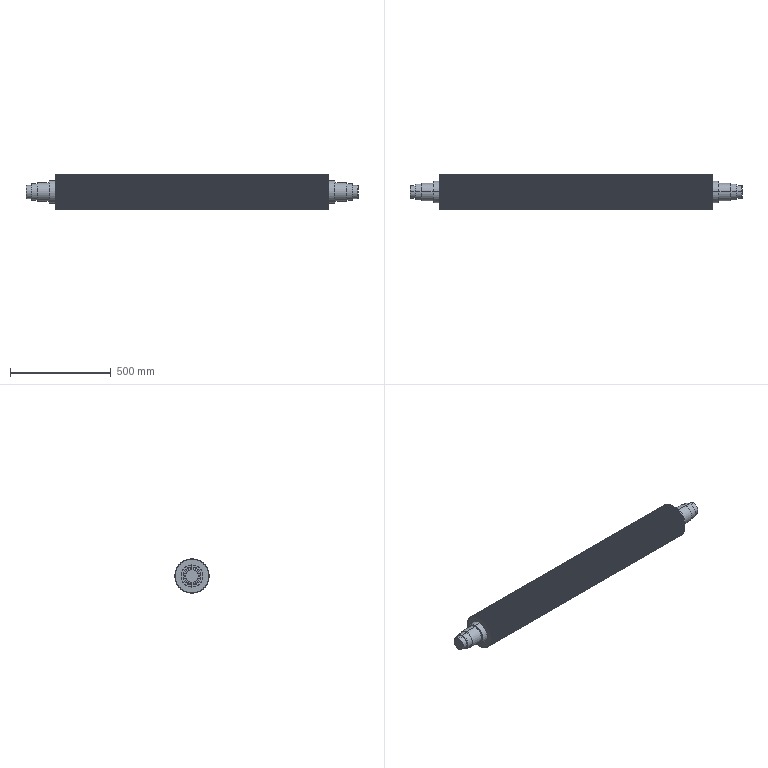Part | SolidWorks | features BaseBody 2 | 2 solids | 617 faces | box 1650 x 169.976 x 169.976 mm | volume 32403710 mm3 | cylinder 591 | cone 16 | plane 10 | commonest cylinder face diameters 1 x288 2 x167 170 x120 65 x4 80 x4 90 x4